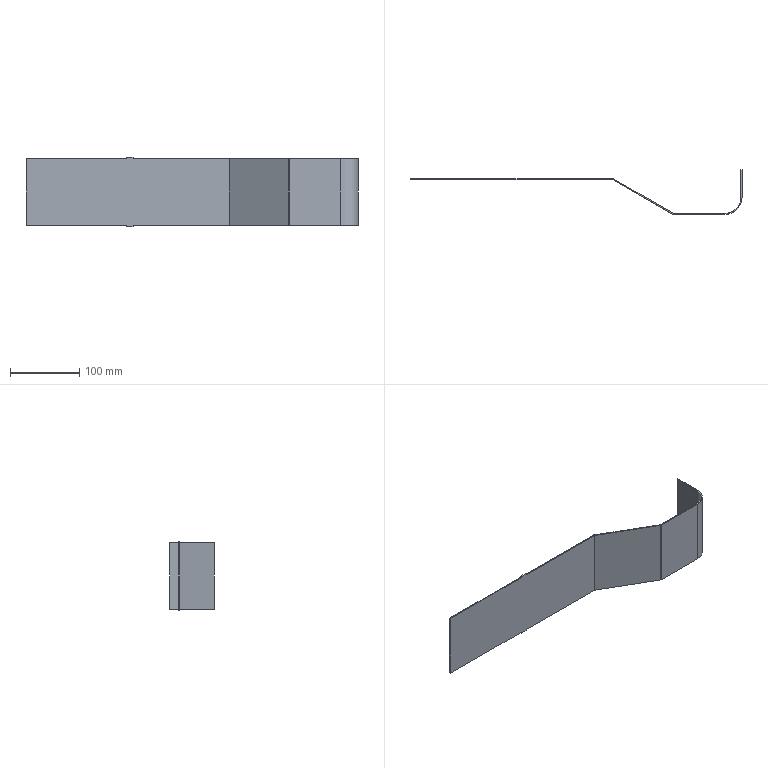Part | STEP file | FHD-021-001-M rack welded part M | 1 solid | 26 faces | box 480.9 x 65 x 100 mm | volume 79687 mm3 | plane 20 | cylinder 6 | commonest cylinder face diameters 0.4 x2 3.4 x2 47 x1 50 x1